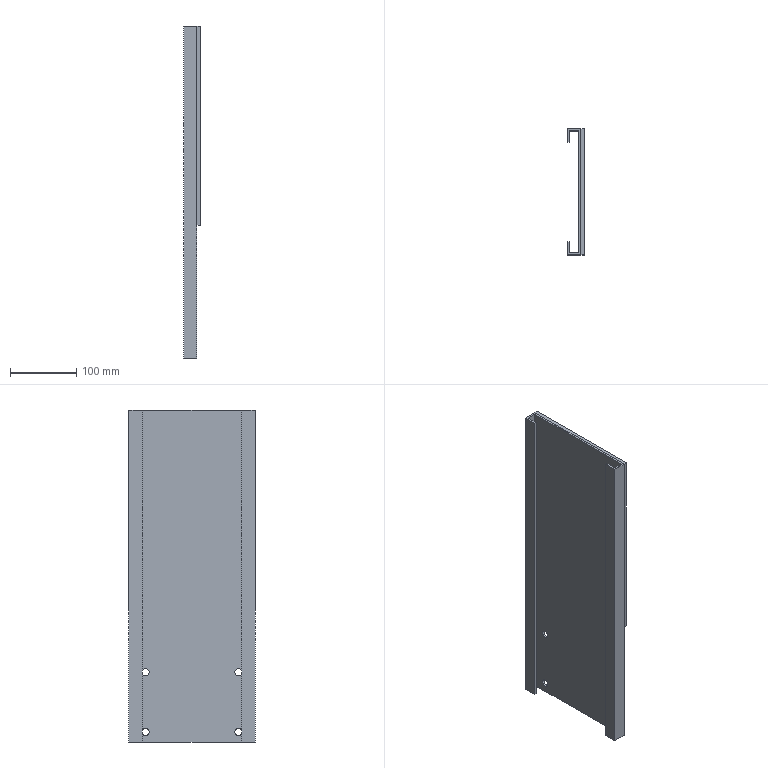Part | STEP file | 2 solids | 28 faces | box 25 x 190 x 500 mm | volume 670860 mm3 | plane 20 | cylinder 8 | commonest cylinder face diameters 11 x8